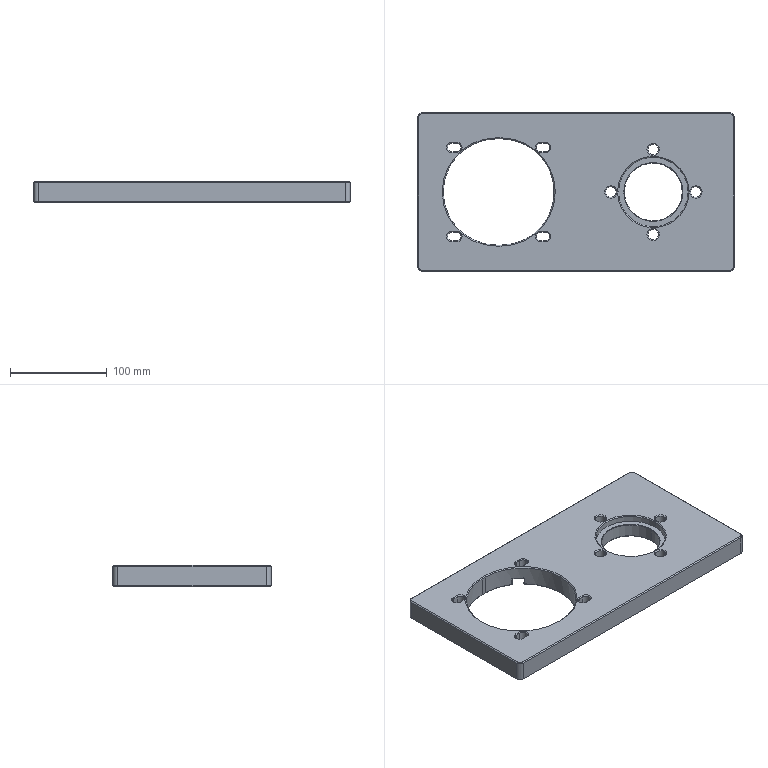NC program | NX | posted with a generic post | part box 328 x 164 x 22 mm
Lines 2823 to 2954 of 5416:
(ZLEVEL_PROFILE_COPY_1_COPY , TOOL : D10JING)
N5626 T09 M6
N5628 G54
N5630 G17 G0 G90 X41.061 Y-32.76 S5000 M3
N5632 G43 Z30. H9
N5634 Z-8.
N5636 G94 G1 X40.889 Y-33.314 F1000.
N5638 G3 X41.11 Y-34.29 R1.
N5640 G2 X36.703 Y-44.362 R6. F1200.
N5642 G1 X28.538
N5644 G3 X26.938 Y-45.962 R1.6
N5646 X28.538 Y-47.562 R1.6
N5648 G1 X39.538
N5650 G3 X41.123 Y-46.182 R1.6
N5652 G2 X50.327 Y-41.971 R6.
N5654 G3 X51.325 Y-42.022 R1.
N5656 G1 X51.853 Y-41.752
N5658 G0 Z30.
N5660 Y41.752
N5662 Z-8.
N5664 G1 X51.325 Y42.022 F1000.
N5666 G3 X50.327 Y41.971 R1.
N5668 G2 X41.123 Y46.182 R6. F1200.
N5670 G3 X39.538 Y47.562 R1.6
N5672 G1 X28.538
N5674 G3 X26.938 Y45.962 R1.6
N5676 X28.538 Y44.362 R1.6
N5678 G1 X36.703
N5680 G2 X41.16 Y34.345 R6.
N5682 G3 X40.952 Y33.367 R1.
N5684 G1 X41.126 Y32.832
N5686 G0 Z30.
N5688 X118.85 Y32.859
N5690 Z-8.
N5692 G1 X119.024 Y33.388 F1000.
N5694 G3 X118.82 Y34.367 R1.
N5696 G2 X123.297 Y44.362 R6. F1200.
N5698 G1 X131.462
N5700 G3 X133.062 Y45.962 R1.6
N5702 X131.462 Y47.562 R1.6
N5704 G1 X120.462
N5706 G3 X118.877 Y46.182 R1.6
N5708 G2 X109.811 Y41.884 R6.001
N5710 G1 X109.68 Y41.969
N5712 X109.663 Y41.978
N5714 G3 X108.664 Y41.944 R1.
N5716 G1 X108.252 Y41.687
N5718 G0 Z30.
N5720 X108.147 Y-41.752
N5722 Z-8.
N5724 G1 X108.675 Y-42.022 F1000.
N5726 G3 X109.673 Y-41.971 R1.
N5728 G2 X118.877 Y-46.182 R6. F1200.
N5730 G3 X120.462 Y-47.562 R1.6
N5732 G1 X131.462
N5734 G3 X133.062 Y-45.962 R1.6
N5736 X131.462 Y-44.362 R1.6
N5738 G1 X123.297
N5740 G2 X118.779 Y-34.413 R6.
N5742 G3 X118.973 Y-33.432 R1.
N5744 G1 X118.797 Y-32.917
N5746 G0 Z30.
(HOLE_MILLING_COPY_1 , TOOL : D10JING)
N5748 X-80. Y44.
N5750 Z0.5
N5752 G1 X-80.462 Y44.876 F1000.
N5754 G3 X-84. Y44. R1.877
N5756 X-84. Y44. Z-1.5 I4. J0. F1200.
N5758 X-84. Y44. Z-3.5 I4. J0.
N5760 X-84. Y44. Z-5.5 I4. J0.
N5762 X-84. Y44. Z-7.5 I4. J0.
N5764 X-84. Y44. Z-9.5 I4. J0.
N5766 X-84. Y44. Z-11.5 I4. J0.
N5768 X-80. Y40. Z-12. R4.
N5770 X-76. Y44. R4.
N5772 X-80. Y40. R-4.
N5774 X-79.124 Y43.538 R1.877
N5776 G1 X-80. Y44.
N5778 G0 Z30.
N5780 X-36. Y0.
N5782 Z0.5
N5784 G1 X-36.462 Y0.876 F1000.
N5786 G3 X-40. Y0. R1.877
N5788 X-40. Y0. Z-1.5 I4. J0. F1200.
N5790 X-40. Y0. Z-3.5 I4. J0.
N5792 X-40. Y0. Z-5.5 I4. J0.
N5794 X-40. Y0. Z-7.5 I4. J0.
N5796 X-40. Y0. Z-9.5 I4. J0.
N5798 X-40. Y0. Z-11.5 I4. J0.
N5800 X-36. Y-4. Z-12. R4.
N5802 X-32. Y0. R4.
N5804 X-36. Y-4. R-4.
N5806 X-35.124 Y-0.462 R1.877
N5808 G1 X-36. Y0.
N5810 G0 Z30.
N5812 X-80. Y-44.
N5814 Z0.5
N5816 G1 X-80.462 Y-43.124 F1000.
N5818 G3 X-84. Y-44. R1.877
N5820 X-84. Y-44. Z-1.5 I4. J0. F1200.
N5822 X-84. Y-44. Z-3.5 I4. J0.
N5824 X-84. Y-44. Z-5.5 I4. J0.
N5826 X-84. Y-44. Z-7.5 I4. J0.
N5828 X-84. Y-44. Z-9.5 I4. J0.
N5830 X-84. Y-44. Z-11.5 I4. J0.
N5832 X-80. Y-48. Z-12. R4.
N5834 X-76. Y-44. R4.
N5836 X-80. Y-48. R-4.
N5838 X-79.124 Y-44.462 R1.877
N5840 G1 X-80. Y-44.
N5842 G0 Z30.
N5844 X-124. Y0.
N5846 Z0.5
N5848 G1 X-124.462 Y0.876 F1000.
N5850 G3 X-128. Y0. R1.877
N5852 X-128. Y0. Z-1.5 I4. J0. F1200.
N5854 X-128. Y0. Z-3.5 I4. J0.
N5856 X-128. Y0. Z-5.5 I4. J0.
N5858 X-128. Y0. Z-7.5 I4. J0.
N5860 X-128. Y0. Z-9.5 I4. J0.
N5862 X-128. Y0. Z-11.5 I4. J0.
N5864 X-124. Y-4. Z-12. R4.
N5866 X-120. Y0. R4.
N5868 X-124. Y-4. R-4.
N5870 X-123.124 Y-0.462 R1.877
N5872 G1 X-124. Y0.
N5874 G0 Z30.
N5876 M5